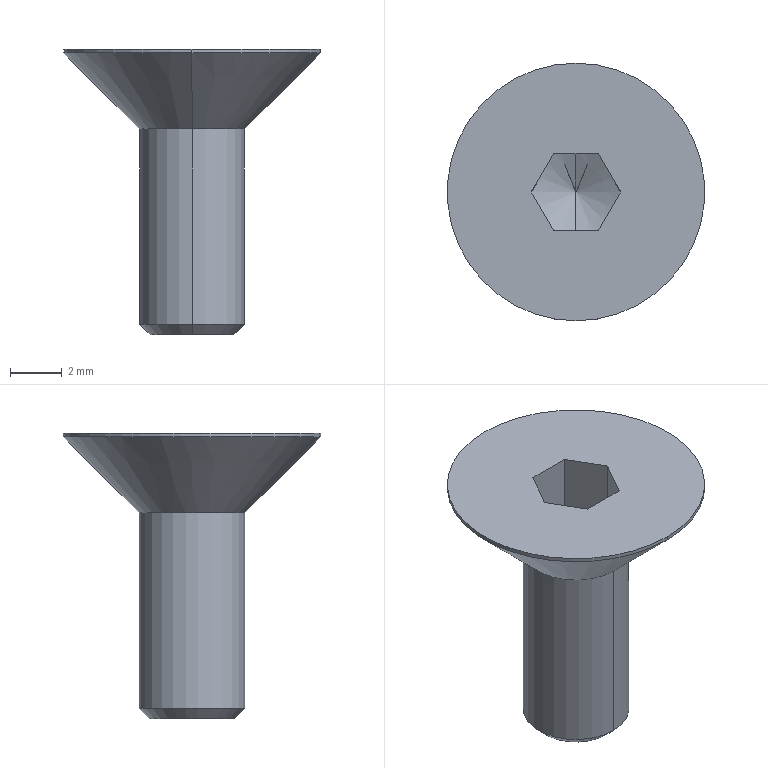Part | STEP file | Flat-head stainless hex socket screw_M5_8 | 1 solid | 24 faces | box 10 x 10 x 11.1 mm | volume 211.569 mm3 | plane 14 | cone 6 | cylinder 4 | commonest cylinder face diameters 4.1 x2 10 x2
STEP:
#1=CARTESIAN_POINT('',(0.,0.,0.));
#2=DIRECTION('',(0.,0.,1.));
#3=DIRECTION('',(1.,0.,0.));
#4=AXIS2_PLACEMENT_3D('',#1,#2,#3);
#5=CARTESIAN_POINT('',(0.,-5.,3.1));
#6=VERTEX_POINT('',#5);
#7=CARTESIAN_POINT('',(0.,5.,3.1));
#8=VERTEX_POINT('',#7);
#9=CARTESIAN_POINT('',(0.,0.,3.1));
#10=DIRECTION('',(0.,0.,1.));
#11=DIRECTION('',(0.,1.,0.));
#12=AXIS2_PLACEMENT_3D('',#9,#10,#11);
#13=CIRCLE('',#12,5.);
#14=CARTESIAN_POINT('',(0.,0.,3.1));
#15=DIRECTION('',(0.,0.,-1.));
#16=DIRECTION('',(0.,1.,0.));
#17=AXIS2_PLACEMENT_3D('',#14,#15,#16);
#18=CYLINDRICAL_SURFACE('',#17,5.);
#19=CARTESIAN_POINT('',(6.283,0.));
#20=DIRECTION('',(-1.,0.));
#21=VECTOR('',#20,1.);
#22=LINE('',#19,#21);
#23=(GEOMETRIC_REPRESENTATION_CONTEXT(2)PARAMETRIC_REPRESENTATION_CONTEXT()REPRESENTATION_CONTEXT('',''));
#24=DEFINITIONAL_REPRESENTATION('',(#22),#23);
#25=PCURVE('',#18,#24);
#26=CARTESIAN_POINT('',(0.,0.,3.1));
#27=DIRECTION('',(0.,0.,1.));
#28=DIRECTION('',(0.,-1.,0.));
#29=AXIS2_PLACEMENT_3D('',#26,#27,#28);
#30=PLANE('',#29);
#31=CARTESIAN_POINT('',(0.,0.));
#32=DIRECTION('',(-1.,0.));
#33=AXIS2_PLACEMENT_2D('',#31,#32);
#34=CIRCLE('',#33,5.);
#35=(GEOMETRIC_REPRESENTATION_CONTEXT(2)PARAMETRIC_REPRESENTATION_CONTEXT()REPRESENTATION_CONTEXT('',''));
#36=DEFINITIONAL_REPRESENTATION('',(#34),#35);
#37=PCURVE('',#30,#36);
#38=SURFACE_CURVE('',#13,(#25,#37),.PCURVE_S1.);
#39=EDGE_CURVE('',#6,#8,#38,.T.);
#40=ORIENTED_EDGE('',*,*,#39,.F.);
#41=CARTESIAN_POINT('',(0.,-5.,2.95));
#42=VERTEX_POINT('',#41);
#43=CARTESIAN_POINT('',(0.,-5.,3.1));
#44=DIRECTION('',(0.,0.,-1.));
#45=VECTOR('',#44,1.);
#46=LINE('',#43,#45);
#47=CARTESIAN_POINT('',(3.142,0.));
#48=DIRECTION('',(0.,1.));
#49=VECTOR('',#48,1.);
#50=LINE('',#47,#49);
#51=(GEOMETRIC_REPRESENTATION_CONTEXT(2)PARAMETRIC_REPRESENTATION_CONTEXT()REPRESENTATION_CONTEXT('',''));
#52=DEFINITIONAL_REPRESENTATION('',(#50),#51);
#53=PCURVE('',#18,#52);
#54=CARTESIAN_POINT('',(0.,0.,3.1));
#55=DIRECTION('',(0.,0.,-1.));
#56=DIRECTION('',(0.,1.,0.));
#57=AXIS2_PLACEMENT_3D('',#54,#55,#56);
#58=CYLINDRICAL_SURFACE('',#57,5.);
#59=CARTESIAN_POINT('',(3.142,0.));
#60=DIRECTION('',(0.,1.));
#61=VECTOR('',#60,1.);
#62=LINE('',#59,#61);
#63=(GEOMETRIC_REPRESENTATION_CONTEXT(2)PARAMETRIC_REPRESENTATION_CONTEXT()REPRESENTATION_CONTEXT('',''));
#64=DEFINITIONAL_REPRESENTATION('',(#62),#63);
#65=PCURVE('',#58,#64);
#66=SURFACE_CURVE('',#46,(#53,#65),.PCURVE_S1.);
#67=EDGE_CURVE('',#6,#42,#66,.T.);
#68=ORIENTED_EDGE('',*,*,#67,.T.);
#69=CARTESIAN_POINT('',(0.,5.,2.95));
#70=VERTEX_POINT('',#69);
#71=CARTESIAN_POINT('',(0.,0.,2.95));
#72=DIRECTION('',(0.,0.,1.));
#73=DIRECTION('',(0.,1.,0.));
#74=AXIS2_PLACEMENT_3D('',#71,#72,#73);
#75=CIRCLE('',#74,5.);
#76=CARTESIAN_POINT('',(6.283,0.15));
#77=DIRECTION('',(-1.,0.));
#78=VECTOR('',#77,1.);
#79=LINE('',#76,#78);
#80=(GEOMETRIC_REPRESENTATION_CONTEXT(2)PARAMETRIC_REPRESENTATION_CONTEXT()REPRESENTATION_CONTEXT('',''));
#81=DEFINITIONAL_REPRESENTATION('',(#79),#80);
#82=PCURVE('',#18,#81);
#83=CARTESIAN_POINT('',(0.,0.,2.95));
#84=DIRECTION('',(0.,0.,1.));
#85=DIRECTION('',(0.,-1.,0.));
#86=AXIS2_PLACEMENT_3D('',#83,#84,#85);
#87=CONICAL_SURFACE('',#86,5.,0.7854);
#88=CARTESIAN_POINT('',(-3.142,0.));
#89=DIRECTION('',(1.,0.));
#90=VECTOR('',#89,1.);
#91=LINE('',#88,#90);
#92=(GEOMETRIC_REPRESENTATION_CONTEXT(2)PARAMETRIC_REPRESENTATION_CONTEXT()REPRESENTATION_CONTEXT('',''));
#93=DEFINITIONAL_REPRESENTATION('',(#91),#92);
#94=PCURVE('',#87,#93);
#95=SURFACE_CURVE('',#75,(#82,#94),.PCURVE_S1.);
#96=EDGE_CURVE('',#42,#70,#95,.T.);
#97=ORIENTED_EDGE('',*,*,#96,.T.);
#98=CARTESIAN_POINT('',(0.,5.,3.1));
#99=DIRECTION('',(0.,0.,-1.));
#100=VECTOR('',#99,1.);
#101=LINE('',#98,#100);
#102=CARTESIAN_POINT('',(0.,0.));
#103=DIRECTION('',(0.,1.));
#104=VECTOR('',#103,1.);
#105=LINE('',#102,#104);
#106=(GEOMETRIC_REPRESENTATION_CONTEXT(2)PARAMETRIC_REPRESENTATION_CONTEXT()REPRESENTATION_CONTEXT('',''));
#107=DEFINITIONAL_REPRESENTATION('',(#105),#106);
#108=PCURVE('',#18,#107);
#109=CARTESIAN_POINT('',(6.283,0.));
#110=DIRECTION('',(0.,1.));
#111=VECTOR('',#110,1.);
#112=LINE('',#109,#111);
#113=(GEOMETRIC_REPRESENTATION_CONTEXT(2)PARAMETRIC_REPRESENTATION_CONTEXT()REPRESENTATION_CONTEXT('',''));
#114=DEFINITIONAL_REPRESENTATION('',(#112),#113);
#115=PCURVE('',#58,#114);
#116=SURFACE_CURVE('',#101,(#108,#115),.PCURVE_S1.);
#117=EDGE_CURVE('',#8,#70,#116,.T.);
#118=ORIENTED_EDGE('',*,*,#117,.F.);
#119=EDGE_LOOP('',(#40,#68,#97,#118));
#120=FACE_BOUND('',#119,.T.);
#121=ADVANCED_FACE('',(#120),#18,.T.);
#122=CARTESIAN_POINT('',(0.,-2.05,0.));
#123=VERTEX_POINT('',#122);
#124=CARTESIAN_POINT('',(0.,2.05,0.));
#125=VERTEX_POINT('',#124);
#126=CARTESIAN_POINT('',(0.,0.,0.));
#127=DIRECTION('',(0.,0.,1.));
#128=DIRECTION('',(1.,0.,0.));
#129=AXIS2_PLACEMENT_3D('',#126,#127,#128);
#130=CIRCLE('',#129,2.05);
#131=CARTESIAN_POINT('',(-4.712,-2.95));
#132=DIRECTION('',(1.,0.));
#133=VECTOR('',#132,1.);
#134=LINE('',#131,#133);
#135=(GEOMETRIC_REPRESENTATION_CONTEXT(2)PARAMETRIC_REPRESENTATION_CONTEXT()REPRESENTATION_CONTEXT('',''));
#136=DEFINITIONAL_REPRESENTATION('',(#134),#135);
#137=PCURVE('',#87,#136);
#138=CARTESIAN_POINT('',(0.,0.,-8.));
#139=DIRECTION('',(0.,0.,1.));
#140=DIRECTION('',(0.,-1.,0.));
#141=AXIS2_PLACEMENT_3D('',#138,#139,#140);
#142=CYLINDRICAL_SURFACE('',#141,2.05);
#143=CARTESIAN_POINT('',(-4.712,8.));
#144=DIRECTION('',(1.,0.));
#145=VECTOR('',#144,1.);
#146=LINE('',#143,#145);
#147=(GEOMETRIC_REPRESENTATION_CONTEXT(2)PARAMETRIC_REPRESENTATION_CONTEXT()REPRESENTATION_CONTEXT('',''));
#148=DEFINITIONAL_REPRESENTATION('',(#146),#147);
#149=PCURVE('',#142,#148);
#150=SURFACE_CURVE('',#130,(#137,#149),.PCURVE_S1.);
#151=EDGE_CURVE('',#123,#125,#150,.T.);
#152=ORIENTED_EDGE('',*,*,#151,.T.);
#153=CARTESIAN_POINT('',(0.,5.,2.95));
#154=DIRECTION('',(0.,0.7071,0.7071));
#155=VECTOR('',#154,1.);
#156=LINE('',#153,#155);
#157=CARTESIAN_POINT('',(3.142,0.));
#158=DIRECTION('',(0.,1.));
#159=VECTOR('',#158,1.);
#160=LINE('',#157,#159);
#161=(GEOMETRIC_REPRESENTATION_CONTEXT(2)PARAMETRIC_REPRESENTATION_CONTEXT()REPRESENTATION_CONTEXT('',''));
#162=DEFINITIONAL_REPRESENTATION('',(#160),#161);
#163=PCURVE('',#87,#162);
#164=CARTESIAN_POINT('',(0.,0.,2.95));
#165=DIRECTION('',(0.,0.,1.));
#166=DIRECTION('',(0.,-1.,0.));
#167=AXIS2_PLACEMENT_3D('',#164,#165,#166);
#168=CONICAL_SURFACE('',#167,5.,0.7854);
#169=CARTESIAN_POINT('',(3.142,0.));
#170=DIRECTION('',(0.,1.));
#171=VECTOR('',#170,1.);
#172=LINE('',#169,#171);
#173=(GEOMETRIC_REPRESENTATION_CONTEXT(2)PARAMETRIC_REPRESENTATION_CONTEXT()REPRESENTATION_CONTEXT('',''));
#174=DEFINITIONAL_REPRESENTATION('',(#172),#173);
#175=PCURVE('',#168,#174);
#176=SURFACE_CURVE('',#156,(#163,#175),.PCURVE_S1.);
#177=EDGE_CURVE('',#125,#70,#176,.T.);
#178=ORIENTED_EDGE('',*,*,#177,.T.);
#179=ORIENTED_EDGE('',*,*,#96,.F.);
#180=CARTESIAN_POINT('',(0.,-5.,2.95));
#181=DIRECTION('',(0.,-0.7071,0.7071));
#182=VECTOR('',#181,1.);
#183=LINE('',#180,#182);
#184=CARTESIAN_POINT('',(0.,0.));
#185=DIRECTION('',(0.,1.));
#186=VECTOR('',#185,1.);
#187=LINE('',#184,#186);
#188=(GEOMETRIC_REPRESENTATION_CONTEXT(2)PARAMETRIC_REPRESENTATION_CONTEXT()REPRESENTATION_CONTEXT('',''));
#189=DEFINITIONAL_REPRESENTATION('',(#187),#188);
#190=PCURVE('',#87,#189);
#191=CARTESIAN_POINT('',(6.283,0.));
#192=DIRECTION('',(0.,1.));
#193=VECTOR('',#192,1.);
#194=LINE('',#191,#193);
#195=(GEOMETRIC_REPRESENTATION_CONTEXT(2)PARAMETRIC_REPRESENTATION_CONTEXT()REPRESENTATION_CONTEXT('',''));
#196=DEFINITIONAL_REPRESENTATION('',(#194),#195);
#197=PCURVE('',#168,#196);
#198=SURFACE_CURVE('',#183,(#190,#197),.PCURVE_S1.);
#199=EDGE_CURVE('',#123,#42,#198,.T.);
#200=ORIENTED_EDGE('',*,*,#199,.F.);
#201=EDGE_LOOP('',(#152,#178,#179,#200));
#202=FACE_BOUND('',#201,.T.);
#203=ADVANCED_FACE('',(#202),#87,.T.);
#204=CARTESIAN_POINT('',(0.,-2.05,-7.59));
#205=VERTEX_POINT('',#204);
#206=CARTESIAN_POINT('',(0.,2.05,-7.59));
#207=VERTEX_POINT('',#206);
#208=CARTESIAN_POINT('',(0.,0.,-7.59));
#209=DIRECTION('',(0.,0.,1.));
#210=DIRECTION('',(0.,-1.,0.));
#211=AXIS2_PLACEMENT_3D('',#208,#209,#210);
#212=CIRCLE('',#211,2.05);
#213=CARTESIAN_POINT('',(0.,0.41));
#214=DIRECTION('',(1.,0.));
#215=VECTOR('',#214,1.);
#216=LINE('',#213,#215);
#217=(GEOMETRIC_REPRESENTATION_CONTEXT(2)PARAMETRIC_REPRESENTATION_CONTEXT()REPRESENTATION_CONTEXT('',''));
#218=DEFINITIONAL_REPRESENTATION('',(#216),#217);
#219=PCURVE('',#142,#218);
#220=CARTESIAN_POINT('',(0.,0.,-7.59));
#221=DIRECTION('',(0.,0.,1.));
#222=DIRECTION('',(0.,-1.,0.));
#223=AXIS2_PLACEMENT_3D('',#220,#221,#222);
#224=CONICAL_SURFACE('',#223,2.05,0.7854);
#225=CARTESIAN_POINT('',(0.,0.));
#226=DIRECTION('',(1.,0.));
#227=VECTOR('',#226,1.);
#228=LINE('',#225,#227);
#229=(GEOMETRIC_REPRESENTATION_CONTEXT(2)PARAMETRIC_REPRESENTATION_CONTEXT()REPRESENTATION_CONTEXT('',''));
#230=DEFINITIONAL_REPRESENTATION('',(#228),#229);
#231=PCURVE('',#224,#230);
#232=SURFACE_CURVE('',#212,(#219,#231),.PCURVE_S1.);
#233=EDGE_CURVE('',#205,#207,#232,.T.);
#234=ORIENTED_EDGE('',*,*,#233,.T.);
#235=CARTESIAN_POINT('',(0.,2.05,-8.));
#236=DIRECTION('',(0.,0.,1.));
#237=VECTOR('',#236,1.);
#238=LINE('',#235,#237);
#239=CARTESIAN_POINT('',(3.142,0.));
#240=DIRECTION('',(0.,1.));
#241=VECTOR('',#240,1.);
#242=LINE('',#239,#241);
#243=(GEOMETRIC_REPRESENTATION_CONTEXT(2)PARAMETRIC_REPRESENTATION_CONTEXT()REPRESENTATION_CONTEXT('',''));
#244=DEFINITIONAL_REPRESENTATION('',(#242),#243);
#245=PCURVE('',#142,#244);
#246=CARTESIAN_POINT('',(0.,0.,-8.));
#247=DIRECTION('',(0.,0.,1.));
#248=DIRECTION('',(0.,-1.,0.));
#249=AXIS2_PLACEMENT_3D('',#246,#247,#248);
#250=CYLINDRICAL_SURFACE('',#249,2.05);
#251=CARTESIAN_POINT('',(3.142,0.));
#252=DIRECTION('',(0.,1.));
#253=VECTOR('',#252,1.);
#254=LINE('',#251,#253);
#255=(GEOMETRIC_REPRESENTATION_CONTEXT(2)PARAMETRIC_REPRESENTATION_CONTEXT()REPRESENTATION_CONTEXT('',''));
#256=DEFINITIONAL_REPRESENTATION('',(#254),#255);
#257=PCURVE('',#250,#256);
#258=SURFACE_CURVE('',#238,(#245,#257),.PCURVE_S1.);
#259=EDGE_CURVE('',#207,#125,#258,.T.);
#260=ORIENTED_EDGE('',*,*,#259,.T.);
#261=ORIENTED_EDGE('',*,*,#151,.F.);
#262=CARTESIAN_POINT('',(0.,-2.05,-8.));
#263=DIRECTION('',(0.,0.,1.));
#264=VECTOR('',#263,1.);
#265=LINE('',#262,#264);
#266=CARTESIAN_POINT('',(0.,0.));
#267=DIRECTION('',(0.,1.));
#268=VECTOR('',#267,1.);
#269=LINE('',#266,#268);
#270=(GEOMETRIC_REPRESENTATION_CONTEXT(2)PARAMETRIC_REPRESENTATION_CONTEXT()REPRESENTATION_CONTEXT('',''));
#271=DEFINITIONAL_REPRESENTATION('',(#269),#270);
#272=PCURVE('',#142,#271);
#273=CARTESIAN_POINT('',(6.283,0.));
#274=DIRECTION('',(0.,1.));
#275=VECTOR('',#274,1.);
#276=LINE('',#273,#275);
#277=(GEOMETRIC_REPRESENTATION_CONTEXT(2)PARAMETRIC_REPRESENTATION_CONTEXT()REPRESENTATION_CONTEXT('',''));
#278=DEFINITIONAL_REPRESENTATION('',(#276),#277);
#279=PCURVE('',#250,#278);
#280=SURFACE_CURVE('',#265,(#272,#279),.PCURVE_S1.);
#281=EDGE_CURVE('',#205,#123,#280,.T.);
#282=ORIENTED_EDGE('',*,*,#281,.F.);
#283=EDGE_LOOP('',(#234,#260,#261,#282));
#284=FACE_BOUND('',#283,.T.);
#285=ADVANCED_FACE('',(#284),#142,.T.);
#286=CARTESIAN_POINT('',(0.,-1.64,-8.));
#287=VERTEX_POINT('',#286);
#288=CARTESIAN_POINT('',(0.,1.64,-8.));
#289=VERTEX_POINT('',#288);
#290=CARTESIAN_POINT('',(0.,0.,-8.));
#291=DIRECTION('',(0.,0.,1.));
#292=DIRECTION('',(0.,-1.,0.));
#293=AXIS2_PLACEMENT_3D('',#290,#291,#292);
#294=CIRCLE('',#293,1.64);
#295=CARTESIAN_POINT('',(0.,-0.41));
#296=DIRECTION('',(1.,0.));
#297=VECTOR('',#296,1.);
#298=LINE('',#295,#297);
#299=(GEOMETRIC_REPRESENTATION_CONTEXT(2)PARAMETRIC_REPRESENTATION_CONTEXT()REPRESENTATION_CONTEXT('',''));
#300=DEFINITIONAL_REPRESENTATION('',(#298),#299);
#301=PCURVE('',#224,#300);
#302=CARTESIAN_POINT('',(0.,0.,-8.));
#303=DIRECTION('',(0.,0.,-1.));
#304=DIRECTION('',(0.,1.,0.));
#305=AXIS2_PLACEMENT_3D('',#302,#303,#304);
#306=PLANE('',#305);
#307=CARTESIAN_POINT('',(-1.64,0.));
#308=CARTESIAN_POINT('',(-1.64,2.841));
#309=CARTESIAN_POINT('',(0.82,1.42));
#310=CARTESIAN_POINT('',(3.28,0.));
#311=CARTESIAN_POINT('',(0.82,-1.42));
#312=CARTESIAN_POINT('',(-1.64,-2.841));
#313=CARTESIAN_POINT('',(-1.64,0.));
#314=(BOUNDED_CURVE()B_SPLINE_CURVE(2,(#307,#308,#309,#310,#311,#312,#313),.UNSPECIFIED.,.T.,.F.)B_SPLINE_CURVE_WITH_KNOTS((1,2,2,2,2,1),(-2.094,0.,2.094,4.189,6.283,8.378),.UNSPECIFIED.)CURVE()GEOMETRIC_REPRESENTATION_ITEM()RATIONAL_B_SPLINE_CURVE((1.,0.5,1.,0.5,1.,0.5,1.))REPRESENTATION_ITEM(''));
#315=(GEOMETRIC_REPRESENTATION_CONTEXT(2)PARAMETRIC_REPRESENTATION_CONTEXT()REPRESENTATION_CONTEXT('',''));
#316=DEFINITIONAL_REPRESENTATION('',(#314),#315);
#317=PCURVE('',#306,#316);
#318=SURFACE_CURVE('',#294,(#301,#317),.PCURVE_S1.);
#319=EDGE_CURVE('',#287,#289,#318,.T.);
#320=ORIENTED_EDGE('',*,*,#319,.T.);
#321=CARTESIAN_POINT('',(0.,2.05,-7.59));
#322=DIRECTION('',(0.,0.7071,0.7071));
#323=VECTOR('',#322,1.);
#324=LINE('',#321,#323);
#325=CARTESIAN_POINT('',(3.142,0.));
#326=DIRECTION('',(0.,1.));
#327=VECTOR('',#326,1.);
#328=LINE('',#325,#327);
#329=(GEOMETRIC_REPRESENTATION_CONTEXT(2)PARAMETRIC_REPRESENTATION_CONTEXT()REPRESENTATION_CONTEXT('',''));
#330=DEFINITIONAL_REPRESENTATION('',(#328),#329);
#331=PCURVE('',#224,#330);
#332=CARTESIAN_POINT('',(0.,0.,-7.59));
#333=DIRECTION('',(0.,0.,1.));
#334=DIRECTION('',(0.,-1.,0.));
#335=AXIS2_PLACEMENT_3D('',#332,#333,#334);
#336=CONICAL_SURFACE('',#335,2.05,0.7854);
#337=CARTESIAN_POINT('',(3.142,0.));
#338=DIRECTION('',(0.,1.));
#339=VECTOR('',#338,1.);
#340=LINE('',#337,#339);
#341=(GEOMETRIC_REPRESENTATION_CONTEXT(2)PARAMETRIC_REPRESENTATION_CONTEXT()REPRESENTATION_CONTEXT('',''));
#342=DEFINITIONAL_REPRESENTATION('',(#340),#341);
#343=PCURVE('',#336,#342);
#344=SURFACE_CURVE('',#324,(#331,#343),.PCURVE_S1.);
#345=EDGE_CURVE('',#289,#207,#344,.T.);
#346=ORIENTED_EDGE('',*,*,#345,.T.);
#347=ORIENTED_EDGE('',*,*,#233,.F.);
#348=CARTESIAN_POINT('',(0.,-2.05,-7.59));
#349=DIRECTION('',(0.,-0.7071,0.7071));
#350=VECTOR('',#349,1.);
#351=LINE('',#348,#350);
#352=CARTESIAN_POINT('',(0.,0.));
#353=DIRECTION('',(0.,1.));
#354=VECTOR('',#353,1.);
#355=LINE('',#352,#354);
#356=(GEOMETRIC_REPRESENTATION_CONTEXT(2)PARAMETRIC_REPRESENTATION_CONTEXT()REPRESENTATION_CONTEXT('',''));
#357=DEFINITIONAL_REPRESENTATION('',(#355),#356);
#358=PCURVE('',#224,#357);
#359=CARTESIAN_POINT('',(6.283,0.));
#360=DIRECTION('',(0.,1.));
#361=VECTOR('',#360,1.);
#362=LINE('',#359,#361);
#363=(GEOMETRIC_REPRESENTATION_CONTEXT(2)PARAMETRIC_REPRESENTATION_CONTEXT()REPRESENTATION_CONTEXT('',''));
#364=DEFINITIONAL_REPRESENTATION('',(#362),#363);
#365=PCURVE('',#336,#364);
#366=SURFACE_CURVE('',#351,(#358,#365),.PCURVE_S1.);
#367=EDGE_CURVE('',#287,#205,#366,.T.);
#368=ORIENTED_EDGE('',*,*,#367,.F.);
#369=EDGE_LOOP('',(#320,#346,#347,#368));
#370=FACE_BOUND('',#369,.T.);
#371=ADVANCED_FACE('',(#370),#224,.T.);
#372=CARTESIAN_POINT('',(-0.866,-1.5,0.));
#373=VERTEX_POINT('',#372);
#374=CARTESIAN_POINT('',(0.,-1.732,0.));
#375=VERTEX_POINT('',#374);
#376=CARTESIAN_POINT('',(0.,0.,0.));
#377=DIRECTION('',(0.,0.,1.));
#378=DIRECTION('',(0.,-1.,0.));
#379=AXIS2_PLACEMENT_3D('',#376,#377,#378);
#380=CIRCLE('',#379,1.732);
#381=CARTESIAN_POINT('',(0.,0.,0.));
#382=DIRECTION('',(0.,0.,1.));
#383=DIRECTION('',(0.,-1.,0.));
#384=AXIS2_PLACEMENT_3D('',#381,#382,#383);
#385=CONICAL_SURFACE('',#384,1.732,1.134);
#386=CARTESIAN_POINT('',(0.,0.));
#387=DIRECTION('',(1.,0.));
#388=VECTOR('',#387,1.);
#389=LINE('',#386,#388);
#390=(GEOMETRIC_REPRESENTATION_CONTEXT(2)PARAMETRIC_REPRESENTATION_CONTEXT()REPRESENTATION_CONTEXT('',''));
#391=DEFINITIONAL_REPRESENTATION('',(#389),#390);
#392=PCURVE('',#385,#391);
#393=CARTESIAN_POINT('',(1.732,0.,0.));
#394=DIRECTION('',(0.,0.,1.));
#395=DIRECTION('',(0.,-1.,0.));
#396=AXIS2_PLACEMENT_3D('',#393,#394,#395);
#397=PLANE('',#396);
#398=CARTESIAN_POINT('',(0.,-1.732));
#399=DIRECTION('',(1.,0.));
#400=AXIS2_PLACEMENT_2D('',#398,#399);
#401=CIRCLE('',#400,1.732);
#402=(GEOMETRIC_REPRESENTATION_CONTEXT(2)PARAMETRIC_REPRESENTATION_CONTEXT()REPRESENTATION_CONTEXT('',''));
#403=DEFINITIONAL_REPRESENTATION('',(#401),#402);
#404=PCURVE('',#397,#403);
#405=SURFACE_CURVE('',#380,(#392,#404),.PCURVE_S1.);
#406=EDGE_CURVE('',#373,#375,#405,.T.);
#407=ORIENTED_EDGE('',*,*,#406,.F.);
#408=CARTESIAN_POINT('',(-1.732,0.,0.));
#409=VERTEX_POINT('',#408);
#410=CARTESIAN_POINT('',(0.,0.,0.));
#411=DIRECTION('',(0.,0.,-1.));
#412=DIRECTION('',(0.,-1.,0.));
#413=AXIS2_PLACEMENT_3D('',#410,#411,#412);
#414=CIRCLE('',#413,1.732);
#415=CARTESIAN_POINT('',(6.283,0.));
#416=DIRECTION('',(-1.,0.));
#417=VECTOR('',#416,1.);
#418=LINE('',#415,#417);
#419=(GEOMETRIC_REPRESENTATION_CONTEXT(2)PARAMETRIC_REPRESENTATION_CONTEXT()REPRESENTATION_CONTEXT('',''));
#420=DEFINITIONAL_REPRESENTATION('',(#418),#419);
#421=PCURVE('',#385,#420);
#422=CARTESIAN_POINT('',(1.732,0.,0.));
#423=DIRECTION('',(0.,0.,1.));
#424=DIRECTION('',(0.,-1.,0.));
#425=AXIS2_PLACEMENT_3D('',#422,#423,#424);
#426=PLANE('',#425);
#427=CARTESIAN_POINT('',(1.732,-1.732));
#428=CARTESIAN_POINT('',(1.732,-4.732));
#429=CARTESIAN_POINT('',(-0.866,-3.232));
#430=CARTESIAN_POINT('',(-3.464,-1.732));
#431=CARTESIAN_POINT('',(-0.866,-0.2321));
#432=CARTESIAN_POINT('',(1.732,1.268));
#433=CARTESIAN_POINT('',(1.732,-1.732));
#434=(BOUNDED_CURVE()B_SPLINE_CURVE(2,(#427,#428,#429,#430,#431,#432,#433),.UNSPECIFIED.,.T.,.F.)B_SPLINE_CURVE_WITH_KNOTS((1,2,2,2,2,1),(-2.094,0.,2.094,4.189,6.283,8.378),.UNSPECIFIED.)CURVE()GEOMETRIC_REPRESENTATION_ITEM()RATIONAL_B_SPLINE_CURVE((1.,0.5,1.,0.5,1.,0.5,1.))REPRESENTATION_ITEM(''));
#435=(GEOMETRIC_REPRESENTATION_CONTEXT(2)PARAMETRIC_REPRESENTATION_CONTEXT()REPRESENTATION_CONTEXT('',''));
#436=DEFINITIONAL_REPRESENTATION('',(#434),#435);
#437=PCURVE('',#426,#436);
#438=SURFACE_CURVE('',#414,(#421,#437),.PCURVE_S1.);
#439=EDGE_CURVE('',#373,#409,#438,.T.);
#440=ORIENTED_EDGE('',*,*,#439,.T.);
#441=CARTESIAN_POINT('',(-0.866,1.5,0.));
#442=VERTEX_POINT('',#441);
#443=CARTESIAN_POINT('',(0.,0.,0.));
#444=DIRECTION('',(0.,0.,-1.));
#445=DIRECTION('',(0.,-1.,0.));
#446=AXIS2_PLACEMENT_3D('',#443,#444,#445);
#447=CIRCLE('',#446,1.732);
#448=CARTESIAN_POINT('',(6.283,0.));
#449=DIRECTION('',(-1.,0.));
#450=VECTOR('',#449,1.);
#451=LINE('',#448,#450);
#452=(GEOMETRIC_REPRESENTATION_CONTEXT(2)PARAMETRIC_REPRESENTATION_CONTEXT()REPRESENTATION_CONTEXT('',''));
#453=DEFINITIONAL_REPRESENTATION('',(#451),#452);
#454=PCURVE('',#385,#453);
#455=CARTESIAN_POINT('',(1.732,0.,0.));
#456=DIRECTION('',(0.,0.,1.));
#457=DIRECTION('',(0.,-1.,0.));
#458=AXIS2_PLACEMENT_3D('',#455,#456,#457);
#459=PLANE('',#458);
#460=CARTESIAN_POINT('',(1.732,-1.732));
#461=CARTESIAN_POINT('',(1.732,-4.732));
#462=CARTESIAN_POINT('',(-0.866,-3.232));
#463=CARTESIAN_POINT('',(-3.464,-1.732));
#464=CARTESIAN_POINT('',(-0.866,-0.2321));
#465=CARTESIAN_POINT('',(1.732,1.268));
#466=CARTESIAN_POINT('',(1.732,-1.732));
#467=(BOUNDED_CURVE()B_SPLINE_CURVE(2,(#460,#461,#462,#463,#464,#465,#466),.UNSPECIFIED.,.T.,.F.)B_SPLINE_CURVE_WITH_KNOTS((1,2,2,2,2,1),(-2.094,0.,2.094,4.189,6.283,8.378),.UNSPECIFIED.)CURVE()GEOMETRIC_REPRESENTATION_ITEM()RATIONAL_B_SPLINE_CURVE((1.,0.5,1.,0.5,1.,0.5,1.))REPRESENTATION_ITEM(''));
#468=(GEOMETRIC_REPRESENTATION_CONTEXT(2)PARAMETRIC_REPRESENTATION_CONTEXT()REPRESENTATION_CONTEXT('',''));
#469=DEFINITIONAL_REPRESENTATION('',(#467),#468);
#470=PCURVE('',#459,#469);
#471=SURFACE_CURVE('',#447,(#454,#470),.PCURVE_S1.);
#472=EDGE_CURVE('',#409,#442,#471,.T.);
#473=ORIENTED_EDGE('',*,*,#472,.T.);
#474=CARTESIAN_POINT('',(0.,1.732,0.));
#475=VERTEX_POINT('',#474);
#476=CARTESIAN_POINT('',(0.,0.,0.));
#477=DIRECTION('',(0.,0.,-1.));
#478=DIRECTION('',(0.,-1.,0.));
#479=AXIS2_PLACEMENT_3D('',#476,#477,#478);
#480=CIRCLE('',#479,1.732);
#481=CARTESIAN_POINT('',(6.283,0.));
#482=DIRECTION('',(-1.,0.));
#483=VECTOR('',#482,1.);
#484=LINE('',#481,#483);
#485=(GEOMETRIC_REPRESENTATION_CONTEXT(2)PARAMETRIC_REPRESENTATION_CONTEXT()REPRESENTATION_CONTEXT('',''));
#486=DEFINITIONAL_REPRESENTATION('',(#484),#485);
#487=PCURVE('',#385,#486);
#488=CARTESIAN_POINT('',(1.732,0.,0.));
#489=DIRECTION('',(0.,0.,1.));
#490=DIRECTION('',(0.,-1.,0.));
#491=AXIS2_PLACEMENT_3D('',#488,#489,#490);
#492=PLANE('',#491);
#493=CARTESIAN_POINT('',(1.732,-1.732));
#494=CARTESIAN_POINT('',(1.732,-4.732));
#495=CARTESIAN_POINT('',(-0.866,-3.232));
#496=CARTESIAN_POINT('',(-3.464,-1.732));
#497=CARTESIAN_POINT('',(-0.866,-0.2321));
#498=CARTESIAN_POINT('',(1.732,1.268));
#499=CARTESIAN_POINT('',(1.732,-1.732));
#500=(BOUNDED_CURVE()B_SPLINE_CURVE(2,(#493,#494,#495,#496,#497,#498,#499),.UNSPECIFIED.,.T.,.F.)B_SPLINE_CURVE_WITH_KNOTS((1,2,2,2,2,1),(-2.094,0.,2.094,4.189,6.283,8.378),.UNSPECIFIED.)CURVE()GEOMETRIC_REPRESENTATION_ITEM()RATIONAL_B_SPLINE_CURVE((1.,0.5,1.,0.5,1.,0.5,1.))REPRESENTATION_ITEM(''));
#501=(GEOMETRIC_REPRESENTATION_CONTEXT(2)PARAMETRIC_REPRESENTATION_CONTEXT()REPRESENTATION_CONTEXT('',''));
#502=DEFINITIONAL_REPRESENTATION('',(#500),#501);
#503=PCURVE('',#492,#502);
#504=SURFACE_CURVE('',#480,(#487,#503),.PCURVE_S1.);
#505=EDGE_CURVE('',#442,#475,#504,.T.);
#506=ORIENTED_EDGE('',*,*,#505,.T.);
#507=CARTESIAN_POINT('',(0.,0.,-0.8077));
#508=VERTEX_POINT('',#507);
#509=CARTESIAN_POINT('',(0.,1.732,0.));
#510=DIRECTION('',(0.,0.9063,0.4226));
#511=VECTOR('',#510,1.);
#512=LINE('',#509,#511);
#513=CARTESIAN_POINT('',(3.142,0.));
#514=DIRECTION('',(0.,1.));
#515=VECTOR('',#514,1.);
#516=LINE('',#513,#515);
#517=(GEOMETRIC_REPRESENTATION_CONTEXT(2)PARAMETRIC_REPRESENTATION_CONTEXT()REPRESENTATION_CONTEXT('',''));
#518=DEFINITIONAL_REPRESENTATION('',(#516),#517);
#519=PCURVE('',#385,#518);
#520=CARTESIAN_POINT('',(0.,0.,0.));
#521=DIRECTION('',(0.,0.,1.));
#522=DIRECTION('',(0.,-1.,0.));
#523=AXIS2_PLACEMENT_3D('',#520,#521,#522);
#524=CONICAL_SURFACE('',#523,1.732,1.134);
#525=CARTESIAN_POINT('',(3.142,0.));
#526=DIRECTION('',(0.,1.));
#527=VECTOR('',#526,1.);
#528=LINE('',#525,#527);
#529=(GEOMETRIC_REPRESENTATION_CONTEXT(2)PARAMETRIC_REPRESENTATION_CONTEXT()REPRESENTATION_CONTEXT('',''));
#530=DEFINITIONAL_REPRESENTATION('',(#528),#529);
#531=PCURVE('',#524,#530);
#532=SURFACE_CURVE('',#512,(#519,#531),.PCURVE_S1.);
#533=EDGE_CURVE('',#508,#475,#532,.T.);
#534=ORIENTED_EDGE('',*,*,#533,.F.);
#535=CARTESIAN_POINT('',(0.,-1.732,0.));
#536=DIRECTION('',(0.,-0.9063,0.4226));
#537=VECTOR('',#536,1.);
#538=LINE('',#535,#537);
#539=CARTESIAN_POINT('',(6.283,0.));
#540=DIRECTION('',(0.,1.));
#541=VECTOR('',#540,1.);
#542=LINE('',#539,#541);
#543=(GEOMETRIC_REPRESENTATION_CONTEXT(2)PARAMETRIC_REPRESENTATION_CONTEXT()REPRESENTATION_CONTEXT('',''));
#544=DEFINITIONAL_REPRESENTATION('',(#542),#543);
#545=PCURVE('',#385,#544);
#546=CARTESIAN_POINT('',(0.,0.));
#547=DIRECTION('',(0.,1.));
#548=VECTOR('',#547,1.);
#549=LINE('',#546,#548);
#550=(GEOMETRIC_REPRESENTATION_CONTEXT(2)PARAMETRIC_REPRESENTATION_CONTEXT()REPRESENTATION_CONTEXT('',''));
#551=DEFINITIONAL_REPRESENTATION('',(#549),#550);
#552=PCURVE('',#524,#551);
#553=SURFACE_CURVE('',#538,(#545,#552),.PCURVE_S1.);
#554=EDGE_CURVE('',#508,#375,#553,.T.);
#555=ORIENTED_EDGE('',*,*,#554,.T.);
#556=EDGE_LOOP('',(#407,#440,#473,#506,#534,#555));
#557=FACE_BOUND('',#556,.F.);
#558=ADVANCED_FACE('',(#557),#385,.F.);
#559=CARTESIAN_POINT('',(0.,0.,3.1));
#560=DIRECTION('',(0.,0.,1.));
#561=DIRECTION('',(0.,1.,0.));
#562=AXIS2_PLACEMENT_3D('',#559,#560,#561);
#563=CIRCLE('',#562,5.);
#564=CARTESIAN_POINT('',(0.,0.));
#565=DIRECTION('',(-1.,0.));
#566=AXIS2_PLACEMENT_2D('',#564,#565);
#567=CIRCLE('',#566,5.);
#568=(GEOMETRIC_REPRESENTATION_CONTEXT(2)PARAMETRIC_REPRESENTATION_CONTEXT()REPRESENTATION_CONTEXT('',''));
#569=DEFINITIONAL_REPRESENTATION('',(#567),#568);
#570=PCURVE('',#30,#569);
#571=CARTESIAN_POINT('',(6.283,0.));
#572=DIRECTION('',(-1.,0.));
#573=VECTOR('',#572,1.);
#574=LINE('',#571,#573);
#575=(GEOMETRIC_REPRESENTATION_CONTEXT(2)PARAMETRIC_REPRESENTATION_CONTEXT()REPRESENTATION_CONTEXT('',''));
#576=DEFINITIONAL_REPRESENTATION('',(#574),#575);
#577=PCURVE('',#58,#576);
#578=SURFACE_CURVE('',#563,(#570,#577),.PCURVE_S1.);
#579=EDGE_CURVE('',#8,#6,#578,.T.);
#580=ORIENTED_EDGE('',*,*,#579,.T.);
#581=ORIENTED_EDGE('',*,*,#39,.T.);
#582=EDGE_LOOP('',(#580,#581));
#583=FACE_BOUND('',#582,.T.);
#584=CARTESIAN_POINT('',(-1.732,0.,3.1));
#585=VERTEX_POINT('',#584);
#586=CARTESIAN_POINT('',(-0.866,1.5,3.1));
#587=VERTEX_POINT('',#586);
#588=CARTESIAN_POINT('',(-0.866,1.5,3.1));
#589=DIRECTION('',(0.5,0.866,0.));
#590=VECTOR('',#589,1.);
#591=LINE('',#588,#590);
#592=CARTESIAN_POINT('',(-1.5,-0.866));
#593=DIRECTION('',(-0.866,0.5));
#594=VECTOR('',#593,1.);
#595=LINE('',#592,#594);
#596=(GEOMETRIC_REPRESENTATION_CONTEXT(2)PARAMETRIC_REPRESENTATION_CONTEXT()REPRESENTATION_CONTEXT('',''));
#597=DEFINITIONAL_REPRESENTATION('',(#595),#596);
#598=PCURVE('',#30,#597);
#599=CARTESIAN_POINT('',(-0.866,1.5,0.));
#600=DIRECTION('',(-0.866,0.5,0.));
#601=DIRECTION('',(-0.5,-0.866,0.));
#602=AXIS2_PLACEMENT_3D('',#599,#600,#601);
#603=PLANE('',#602);
#604=CARTESIAN_POINT('',(0.,3.1));
#605=DIRECTION('',(-1.,0.));
#606=VECTOR('',#605,1.);
#607=LINE('',#604,#606);
#608=(GEOMETRIC_REPRESENTATION_CONTEXT(2)PARAMETRIC_REPRESENTATION_CONTEXT()REPRESENTATION_CONTEXT('',''));
#609=DEFINITIONAL_REPRESENTATION('',(#607),#608);
#610=PCURVE('',#603,#609);
#611=SURFACE_CURVE('',#591,(#598,#610),.PCURVE_S1.);
#612=EDGE_CURVE('',#585,#587,#611,.T.);
#613=ORIENTED_EDGE('',*,*,#612,.T.);
#614=CARTESIAN_POINT('',(0.866,1.5,3.1));
#615=VERTEX_POINT('',#614);
#616=CARTESIAN_POINT('',(0.,1.5,3.1));
#617=DIRECTION('',(1.,0.,0.));
#618=VECTOR('',#617,1.);
#619=LINE('',#616,#618);
#620=CARTESIAN_POINT('',(-1.5,0.));
#621=DIRECTION('',(0.,1.));
#622=VECTOR('',#621,1.);
#623=LINE('',#620,#622);
#624=(GEOMETRIC_REPRESENTATION_CONTEXT(2)PARAMETRIC_REPRESENTATION_CONTEXT()REPRESENTATION_CONTEXT('',''));
#625=DEFINITIONAL_REPRESENTATION('',(#623),#624);
#626=PCURVE('',#30,#625);
#627=CARTESIAN_POINT('',(0.866,1.5,0.));
#628=DIRECTION('',(0.,1.,0.));
#629=DIRECTION('',(-1.,0.,0.));
#630=AXIS2_PLACEMENT_3D('',#627,#628,#629);
#631=PLANE('',#630);
#632=CARTESIAN_POINT('',(0.866,3.1));
#633=DIRECTION('',(-1.,0.));
#634=VECTOR('',#633,1.);
#635=LINE('',#632,#634);
#636=(GEOMETRIC_REPRESENTATION_CONTEXT(2)PARAMETRIC_REPRESENTATION_CONTEXT()REPRESENTATION_CONTEXT('',''));
#637=DEFINITIONAL_REPRESENTATION('',(#635),#636);
#638=PCURVE('',#631,#637);
#639=SURFACE_CURVE('',#619,(#626,#638),.PCURVE_S1.);
#640=EDGE_CURVE('',#587,#615,#639,.T.);
#641=ORIENTED_EDGE('',*,*,#640,.T.);
#642=CARTESIAN_POINT('',(1.732,0.,3.1));
#643=VERTEX_POINT('',#642);
#644=CARTESIAN_POINT('',(1.732,0.,3.1));
#645=DIRECTION('',(0.5,-0.866,0.));
#646=VECTOR('',#645,1.);
#647=LINE('',#644,#646);
#648=CARTESIAN_POINT('',(0.,1.732));
#649=DIRECTION('',(0.866,0.5));
#650=VECTOR('',#649,1.);
#651=LINE('',#648,#650);
#652=(GEOMETRIC_REPRESENTATION_CONTEXT(2)PARAMETRIC_REPRESENTATION_CONTEXT()REPRESENTATION_CONTEXT('',''));
#653=DEFINITIONAL_REPRESENTATION('',(#651),#652);
#654=PCURVE('',#30,#653);
#655=CARTESIAN_POINT('',(1.732,0.,0.));
#656=DIRECTION('',(0.866,0.5,0.));
#657=DIRECTION('',(-0.5,0.866,0.));
#658=AXIS2_PLACEMENT_3D('',#655,#656,#657);
#659=PLANE('',#658);
#660=CARTESIAN_POINT('',(0.,3.1));
#661=DIRECTION('',(-1.,0.));
#662=VECTOR('',#661,1.);
#663=LINE('',#660,#662);
#664=(GEOMETRIC_REPRESENTATION_CONTEXT(2)PARAMETRIC_REPRESENTATION_CONTEXT()REPRESENTATION_CONTEXT('',''));
#665=DEFINITIONAL_REPRESENTATION('',(#663),#664);
#666=PCURVE('',#659,#665);
#667=SURFACE_CURVE('',#647,(#654,#666),.PCURVE_S1.);
#668=EDGE_CURVE('',#615,#643,#667,.T.);
#669=ORIENTED_EDGE('',*,*,#668,.T.);
#670=CARTESIAN_POINT('',(0.866,-1.5,3.1));
#671=VERTEX_POINT('',#670);
#672=CARTESIAN_POINT('',(0.866,-1.5,3.1));
#673=DIRECTION('',(-0.5,-0.866,0.));
#674=VECTOR('',#673,1.);
#675=LINE('',#672,#674);
#676=CARTESIAN_POINT('',(1.5,0.866));
#677=DIRECTION('',(0.866,-0.5));
#678=VECTOR('',#677,1.);
#679=LINE('',#676,#678);
#680=(GEOMETRIC_REPRESENTATION_CONTEXT(2)PARAMETRIC_REPRESENTATION_CONTEXT()REPRESENTATION_CONTEXT('',''));
#681=DEFINITIONAL_REPRESENTATION('',(#679),#680);
#682=PCURVE('',#30,#681);
#683=CARTESIAN_POINT('',(0.866,-1.5,0.));
#684=DIRECTION('',(0.866,-0.5,0.));
#685=DIRECTION('',(0.5,0.866,0.));
#686=AXIS2_PLACEMENT_3D('',#683,#684,#685);
#687=PLANE('',#686);
#688=CARTESIAN_POINT('',(0.,3.1));
#689=DIRECTION('',(-1.,0.));
#690=VECTOR('',#689,1.);
#691=LINE('',#688,#690);
#692=(GEOMETRIC_REPRESENTATION_CONTEXT(2)PARAMETRIC_REPRESENTATION_CONTEXT()REPRESENTATION_CONTEXT('',''));
#693=DEFINITIONAL_REPRESENTATION('',(#691),#692);
#694=PCURVE('',#687,#693);
#695=SURFACE_CURVE('',#675,(#682,#694),.PCURVE_S1.);
#696=EDGE_CURVE('',#643,#671,#695,.T.);
#697=ORIENTED_EDGE('',*,*,#696,.T.);
#698=CARTESIAN_POINT('',(-0.866,-1.5,3.1));
#699=VERTEX_POINT('',#698);
#700=CARTESIAN_POINT('',(-0.866,-1.5,3.1));
#701=DIRECTION('',(-1.,0.,0.));
#702=VECTOR('',#701,1.);
#703=LINE('',#700,#702);
#704=CARTESIAN_POINT('',(1.5,-0.866));
#705=DIRECTION('',(0.,-1.));
#706=VECTOR('',#705,1.);
#707=LINE('',#704,#706);
#708=(GEOMETRIC_REPRESENTATION_CONTEXT(2)PARAMETRIC_REPRESENTATION_CONTEXT()REPRESENTATION_CONTEXT('',''));
#709=DEFINITIONAL_REPRESENTATION('',(#707),#708);
#710=PCURVE('',#30,#709);
#711=CARTESIAN_POINT('',(-0.866,-1.5,0.));
#712=DIRECTION('',(0.,-1.,0.));
#713=DIRECTION('',(1.,0.,0.));
#714=AXIS2_PLACEMENT_3D('',#711,#712,#713);
#715=PLANE('',#714);
#716=CARTESIAN_POINT('',(0.,3.1));
#717=DIRECTION('',(-1.,0.));
#718=VECTOR('',#717,1.);
#719=LINE('',#716,#718);
#720=(GEOMETRIC_REPRESENTATION_CONTEXT(2)PARAMETRIC_REPRESENTATION_CONTEXT()REPRESENTATION_CONTEXT('',''));
#721=DEFINITIONAL_REPRESENTATION('',(#719),#720);
#722=PCURVE('',#715,#721);
#723=SURFACE_CURVE('',#703,(#710,#722),.PCURVE_S1.);
#724=EDGE_CURVE('',#671,#699,#723,.T.);
#725=ORIENTED_EDGE('',*,*,#724,.T.);
#726=CARTESIAN_POINT('',(-1.732,0.,3.1));
#727=DIRECTION('',(-0.5,0.866,0.));
#728=VECTOR('',#727,1.);
#729=LINE('',#726,#728);
#730=CARTESIAN_POINT('',(0.,-1.732));
#731=DIRECTION('',(-0.866,-0.5));
#732=VECTOR('',#731,1.);
#733=LINE('',#730,#732);
#734=(GEOMETRIC_REPRESENTATION_CONTEXT(2)PARAMETRIC_REPRESENTATION_CONTEXT()REPRESENTATION_CONTEXT('',''));
#735=DEFINITIONAL_REPRESENTATION('',(#733),#734);
#736=PCURVE('',#30,#735);
#737=CARTESIAN_POINT('',(-1.732,0.,0.));
#738=DIRECTION('',(-0.866,-0.5,0.));
#739=DIRECTION('',(0.5,-0.866,0.));
#740=AXIS2_PLACEMENT_3D('',#737,#738,#739);
#741=PLANE('',#740);
#742=CARTESIAN_POINT('',(0.,3.1));
#743=DIRECTION('',(-1.,0.));
#744=VECTOR('',#743,1.);
#745=LINE('',#742,#744);
#746=(GEOMETRIC_REPRESENTATION_CONTEXT(2)PARAMETRIC_REPRESENTATION_CONTEXT()REPRESENTATION_CONTEXT('',''));
#747=DEFINITIONAL_REPRESENTATION('',(#745),#746);
#748=PCURVE('',#741,#747);
#749=SURFACE_CURVE('',#729,(#736,#748),.PCURVE_S1.);
#750=EDGE_CURVE('',#699,#585,#749,.T.);
#751=ORIENTED_EDGE('',*,*,#750,.T.);
#752=EDGE_LOOP('',(#613,#641,#669,#697,#725,#751));
#753=FACE_BOUND('',#752,.T.);
#754=ADVANCED_FACE('',(#583,#753),#30,.T.);
#755=ORIENTED_EDGE('',*,*,#67,.F.);
#756=ORIENTED_EDGE('',*,*,#579,.F.);
#757=ORIENTED_EDGE('',*,*,#117,.T.);
#758=CARTESIAN_POINT('',(0.,0.,2.95));
#759=DIRECTION('',(0.,0.,1.));
#760=DIRECTION('',(0.,1.,0.));
#761=AXIS2_PLACEMENT_3D('',#758,#759,#760);
#762=CIRCLE('',#761,5.);
#763=CARTESIAN_POINT('',(6.283,0.15));
#764=DIRECTION('',(-1.,0.));
#765=VECTOR('',#764,1.);
#766=LINE('',#763,#765);
#767=(GEOMETRIC_REPRESENTATION_CONTEXT(2)PARAMETRIC_REPRESENTATION_CONTEXT()REPRESENTATION_CONTEXT('',''));
#768=DEFINITIONAL_REPRESENTATION('',(#766),#767);
#769=PCURVE('',#58,#768);
#770=CARTESIAN_POINT('',(3.142,0.));
#771=DIRECTION('',(1.,0.));
#772=VECTOR('',#771,1.);
#773=LINE('',#770,#772);
#774=(GEOMETRIC_REPRESENTATION_CONTEXT(2)PARAMETRIC_REPRESENTATION_CONTEXT()REPRESENTATION_CONTEXT('',''));
#775=DEFINITIONAL_REPRESENTATION('',(#773),#774);
#776=PCURVE('',#168,#775);
#777=SURFACE_CURVE('',#762,(#769,#776),.PCURVE_S1.);
#778=EDGE_CURVE('',#70,#42,#777,.T.);
#779=ORIENTED_EDGE('',*,*,#778,.T.);
#780=EDGE_LOOP('',(#755,#756,#757,#779));
#781=FACE_BOUND('',#780,.T.);
#782=ADVANCED_FACE('',(#781),#58,.T.);
#783=CARTESIAN_POINT('',(-0.866,1.5,0.));
#784=DIRECTION('',(0.,0.,1.));
#785=VECTOR('',#784,1.);
#786=LINE('',#783,#785);
#787=CARTESIAN_POINT('',(1.732,0.));
#788=DIRECTION('',(0.,1.));
#789=VECTOR('',#788,1.);
#790=LINE('',#787,#789);
#791=(GEOMETRIC_REPRESENTATION_CONTEXT(2)PARAMETRIC_REPRESENTATION_CONTEXT()REPRESENTATION_CONTEXT('',''));
#792=DEFINITIONAL_REPRESENTATION('',(#790),#791);
#793=PCURVE('',#631,#792);
#794=CARTESIAN_POINT('',(0.,0.));
#795=DIRECTION('',(0.,1.));
#796=VECTOR('',#795,1.);
#797=LINE('',#794,#796);
#798=(GEOMETRIC_REPRESENTATION_CONTEXT(2)PARAMETRIC_REPRESENTATION_CONTEXT()REPRESENTATION_CONTEXT('',''));
#799=DEFINITIONAL_REPRESENTATION('',(#797),#798);
#800=PCURVE('',#603,#799);
#801=SURFACE_CURVE('',#786,(#793,#800),.PCURVE_S1.);
#802=EDGE_CURVE('',#442,#587,#801,.T.);
#803=ORIENTED_EDGE('',*,*,#802,.F.);
#804=CARTESIAN_POINT('',(0.866,1.5,0.));
#805=VERTEX_POINT('',#804);
#806=CARTESIAN_POINT('',(1.732,1.5,0.));
#807=DIRECTION('',(1.,0.,0.));
#808=VECTOR('',#807,1.);
#809=LINE('',#806,#808);
#810=CARTESIAN_POINT('',(-0.866,0.));
#811=DIRECTION('',(-1.,0.));
#812=VECTOR('',#811,1.);
#813=LINE('',#810,#812);
#814=(GEOMETRIC_REPRESENTATION_CONTEXT(2)PARAMETRIC_REPRESENTATION_CONTEXT()REPRESENTATION_CONTEXT('',''));
#815=DEFINITIONAL_REPRESENTATION('',(#813),#814);
#816=PCURVE('',#631,#815);
#817=CARTESIAN_POINT('',(-1.5,0.));
#818=DIRECTION('',(0.,1.));
#819=VECTOR('',#818,1.);
#820=LINE('',#817,#819);
#821=(GEOMETRIC_REPRESENTATION_CONTEXT(2)PARAMETRIC_REPRESENTATION_CONTEXT()REPRESENTATION_CONTEXT('',''));
#822=DEFINITIONAL_REPRESENTATION('',(#820),#821);
#823=PCURVE('',#492,#822);
#824=SURFACE_CURVE('',#809,(#816,#823),.PCURVE_S1.);
#825=EDGE_CURVE('',#442,#805,#824,.T.);
#826=ORIENTED_EDGE('',*,*,#825,.T.);
#827=CARTESIAN_POINT('',(0.866,1.5,0.));
#828=DIRECTION('',(0.,0.,-1.));
#829=VECTOR('',#828,1.);
#830=LINE('',#827,#829);
#831=CARTESIAN_POINT('',(0.,0.));
#832=DIRECTION('',(0.,-1.));
#833=VECTOR('',#832,1.);
#834=LINE('',#831,#833);
#835=(GEOMETRIC_REPRESENTATION_CONTEXT(2)PARAMETRIC_REPRESENTATION_CONTEXT()REPRESENTATION_CONTEXT('',''));
#836=DEFINITIONAL_REPRESENTATION('',(#834),#835);
#837=PCURVE('',#631,#836);
#838=CARTESIAN_POINT('',(1.732,0.));
#839=DIRECTION('',(0.,-1.));
#840=VECTOR('',#839,1.);
#841=LINE('',#838,#840);
#842=(GEOMETRIC_REPRESENTATION_CONTEXT(2)PARAMETRIC_REPRESENTATION_CONTEXT()REPRESENTATION_CONTEXT('',''));
#843=DEFINITIONAL_REPRESENTATION('',(#841),#842);
#844=PCURVE('',#659,#843);
#845=SURFACE_CURVE('',#830,(#837,#844),.PCURVE_S1.);
#846=EDGE_CURVE('',#615,#805,#845,.T.);
#847=ORIENTED_EDGE('',*,*,#846,.F.);
#848=ORIENTED_EDGE('',*,*,#640,.F.);
#849=EDGE_LOOP('',(#803,#826,#847,#848));
#850=FACE_BOUND('',#849,.T.);
#851=ADVANCED_FACE('',(#850),#631,.F.);
#852=ORIENTED_EDGE('',*,*,#177,.F.);
#853=CARTESIAN_POINT('',(0.,0.,0.));
#854=DIRECTION('',(0.,0.,1.));
#855=DIRECTION('',(1.,0.,0.));
#856=AXIS2_PLACEMENT_3D('',#853,#854,#855);
#857=CIRCLE('',#856,2.05);
#858=CARTESIAN_POINT('',(1.571,-2.95));
#859=DIRECTION('',(1.,0.));
#860=VECTOR('',#859,1.);
#861=LINE('',#858,#860);
#862=(GEOMETRIC_REPRESENTATION_CONTEXT(2)PARAMETRIC_REPRESENTATION_CONTEXT()REPRESENTATION_CONTEXT('',''));
#863=DEFINITIONAL_REPRESENTATION('',(#861),#862);
#864=PCURVE('',#168,#863);
#865=CARTESIAN_POINT('',(1.571,8.));
#866=DIRECTION('',(1.,0.));
#867=VECTOR('',#866,1.);
#868=LINE('',#865,#867);
#869=(GEOMETRIC_REPRESENTATION_CONTEXT(2)PARAMETRIC_REPRESENTATION_CONTEXT()REPRESENTATION_CONTEXT('',''));
#870=DEFINITIONAL_REPRESENTATION('',(#868),#869);
#871=PCURVE('',#250,#870);
#872=SURFACE_CURVE('',#857,(#864,#871),.PCURVE_S1.);
#873=EDGE_CURVE('',#125,#123,#872,.T.);
#874=ORIENTED_EDGE('',*,*,#873,.T.);
#875=ORIENTED_EDGE('',*,*,#199,.T.);
#876=ORIENTED_EDGE('',*,*,#778,.F.);
#877=EDGE_LOOP('',(#852,#874,#875,#876));
#878=FACE_BOUND('',#877,.T.);
#879=ADVANCED_FACE('',(#878),#168,.T.);
#880=CARTESIAN_POINT('',(-1.732,0.,0.));
#881=DIRECTION('',(0.,0.,1.));
#882=VECTOR('',#881,1.);
#883=LINE('',#880,#882);
#884=CARTESIAN_POINT('',(1.732,0.));
#885=DIRECTION('',(0.,1.));
#886=VECTOR('',#885,1.);
#887=LINE('',#884,#886);
#888=(GEOMETRIC_REPRESENTATION_CONTEXT(2)PARAMETRIC_REPRESENTATION_CONTEXT()REPRESENTATION_CONTEXT('',''));
#889=DEFINITIONAL_REPRESENTATION('',(#887),#888);
#890=PCURVE('',#603,#889);
#891=CARTESIAN_POINT('',(0.,0.));
#892=DIRECTION('',(0.,1.));
#893=VECTOR('',#892,1.);
#894=LINE('',#891,#893);
#895=(GEOMETRIC_REPRESENTATION_CONTEXT(2)PARAMETRIC_REPRESENTATION_CONTEXT()REPRESENTATION_CONTEXT('',''));
#896=DEFINITIONAL_REPRESENTATION('',(#894),#895);
#897=PCURVE('',#741,#896);
#898=SURFACE_CURVE('',#883,(#890,#897),.PCURVE_S1.);
#899=EDGE_CURVE('',#409,#585,#898,.T.);
#900=ORIENTED_EDGE('',*,*,#899,.F.);
#901=CARTESIAN_POINT('',(-1.732,0.,0.));
#902=DIRECTION('',(0.5,0.866,0.));
#903=VECTOR('',#902,1.);
#904=LINE('',#901,#903);
#905=CARTESIAN_POINT('',(1.732,0.));
#906=DIRECTION('',(-1.,0.));
#907=VECTOR('',#906,1.);
#908=LINE('',#905,#907);
#909=(GEOMETRIC_REPRESENTATION_CONTEXT(2)PARAMETRIC_REPRESENTATION_CONTEXT()REPRESENTATION_CONTEXT('',''));
#910=DEFINITIONAL_REPRESENTATION('',(#908),#909);
#911=PCURVE('',#603,#910);
#912=CARTESIAN_POINT('',(0.,-3.464));
#913=DIRECTION('',(-0.866,0.5));
#914=VECTOR('',#913,1.);
#915=LINE('',#912,#914);
#916=(GEOMETRIC_REPRESENTATION_CONTEXT(2)PARAMETRIC_REPRESENTATION_CONTEXT()REPRESENTATION_CONTEXT('',''));
#917=DEFINITIONAL_REPRESENTATION('',(#915),#916);
#918=PCURVE('',#459,#917);
#919=SURFACE_CURVE('',#904,(#911,#918),.PCURVE_S1.);
#920=EDGE_CURVE('',#409,#442,#919,.T.);
#921=ORIENTED_EDGE('',*,*,#920,.T.);
#922=ORIENTED_EDGE('',*,*,#802,.T.);
#923=ORIENTED_EDGE('',*,*,#612,.F.);
#924=EDGE_LOOP('',(#900,#921,#922,#923));
#925=FACE_BOUND('',#924,.T.);
#926=ADVANCED_FACE('',(#925),#603,.F.);
#927=ORIENTED_EDGE('',*,*,#846,.T.);
#928=CARTESIAN_POINT('',(1.732,0.,0.));
#929=VERTEX_POINT('',#928);
#930=CARTESIAN_POINT('',(0.866,1.5,0.));
#931=DIRECTION('',(0.5,-0.866,0.));
#932=VECTOR('',#931,1.);
#933=LINE('',#930,#932);
#934=CARTESIAN_POINT('',(1.732,0.));
#935=DIRECTION('',(-1.,0.));
#936=VECTOR('',#935,1.);
#937=LINE('',#934,#936);
#938=(GEOMETRIC_REPRESENTATION_CONTEXT(2)PARAMETRIC_REPRESENTATION_CONTEXT()REPRESENTATION_CONTEXT('',''));
#939=DEFINITIONAL_REPRESENTATION('',(#937),#938);
#940=PCURVE('',#659,#939);
#941=CARTESIAN_POINT('',(1.732,0.,0.));
#942=DIRECTION('',(0.,0.,1.));
#943=DIRECTION('',(0.,-1.,0.));
#944=AXIS2_PLACEMENT_3D('',#941,#942,#943);
#945=PLANE('',#944);
#946=CARTESIAN_POINT('',(-1.5,-0.866));
#947=DIRECTION('',(0.866,0.5));
#948=VECTOR('',#947,1.);
#949=LINE('',#946,#948);
#950=(GEOMETRIC_REPRESENTATION_CONTEXT(2)PARAMETRIC_REPRESENTATION_CONTEXT()REPRESENTATION_CONTEXT('',''));
#951=DEFINITIONAL_REPRESENTATION('',(#949),#950);
#952=PCURVE('',#945,#951);
#953=SURFACE_CURVE('',#933,(#940,#952),.PCURVE_S1.);
#954=EDGE_CURVE('',#805,#929,#953,.T.);
#955=ORIENTED_EDGE('',*,*,#954,.T.);
#956=CARTESIAN_POINT('',(1.732,0.,0.));
#957=DIRECTION('',(0.,0.,-1.));
#958=VECTOR('',#957,1.);
#959=LINE('',#956,#958);
#960=CARTESIAN_POINT('',(0.,0.));
#961=DIRECTION('',(0.,-1.));
#962=VECTOR('',#961,1.);
#963=LINE('',#960,#962);
#964=(GEOMETRIC_REPRESENTATION_CONTEXT(2)PARAMETRIC_REPRESENTATION_CONTEXT()REPRESENTATION_CONTEXT('',''));
#965=DEFINITIONAL_REPRESENTATION('',(#963),#964);
#966=PCURVE('',#659,#965);
#967=CARTESIAN_POINT('',(1.732,0.));
#968=DIRECTION('',(0.,-1.));
#969=VECTOR('',#968,1.);
#970=LINE('',#967,#969);
#971=(GEOMETRIC_REPRESENTATION_CONTEXT(2)PARAMETRIC_REPRESENTATION_CONTEXT()REPRESENTATION_CONTEXT('',''));
#972=DEFINITIONAL_REPRESENTATION('',(#970),#971);
#973=PCURVE('',#687,#972);
#974=SURFACE_CURVE('',#959,(#966,#973),.PCURVE_S1.);
#975=EDGE_CURVE('',#643,#929,#974,.T.);
#976=ORIENTED_EDGE('',*,*,#975,.F.);
#977=ORIENTED_EDGE('',*,*,#668,.F.);
#978=EDGE_LOOP('',(#927,#955,#976,#977));
#979=FACE_BOUND('',#978,.T.);
#980=ADVANCED_FACE('',(#979),#659,.F.);
#981=ORIENTED_EDGE('',*,*,#259,.F.);
#982=CARTESIAN_POINT('',(0.,0.,-7.59));
#983=DIRECTION('',(0.,0.,1.));
#984=DIRECTION('',(0.,-1.,0.));
#985=AXIS2_PLACEMENT_3D('',#982,#983,#984);
#986=CIRCLE('',#985,2.05);
#987=CARTESIAN_POINT('',(0.,0.41));
#988=DIRECTION('',(1.,0.));
#989=VECTOR('',#988,1.);
#990=LINE('',#987,#989);
#991=(GEOMETRIC_REPRESENTATION_CONTEXT(2)PARAMETRIC_REPRESENTATION_CONTEXT()REPRESENTATION_CONTEXT('',''));
#992=DEFINITIONAL_REPRESENTATION('',(#990),#991);
#993=PCURVE('',#250,#992);
#994=CARTESIAN_POINT('',(0.,0.));
#995=DIRECTION('',(1.,0.));
#996=VECTOR('',#995,1.);
#997=LINE('',#994,#996);
#998=(GEOMETRIC_REPRESENTATION_CONTEXT(2)PARAMETRIC_REPRESENTATION_CONTEXT()REPRESENTATION_CONTEXT('',''));
#999=DEFINITIONAL_REPRESENTATION('',(#997),#998);
#1000=PCURVE('',#336,#999);
#1001=SURFACE_CURVE('',#986,(#993,#1000),.PCURVE_S1.);
#1002=EDGE_CURVE('',#207,#205,#1001,.T.);
#1003=ORIENTED_EDGE('',*,*,#1002,.T.);
#1004=ORIENTED_EDGE('',*,*,#281,.T.);
#1005=ORIENTED_EDGE('',*,*,#873,.F.);
#1006=EDGE_LOOP('',(#981,#1003,#1004,#1005));
#1007=FACE_BOUND('',#1006,.T.);
#1008=ADVANCED_FACE('',(#1007),#250,.T.);
#1009=CARTESIAN_POINT('',(-0.866,-1.5,0.));
#1010=DIRECTION('',(0.,0.,1.));
#1011=VECTOR('',#1010,1.);
#1012=LINE('',#1009,#1011);
#1013=CARTESIAN_POINT('',(1.732,0.));
#1014=DIRECTION('',(0.,1.));
#1015=VECTOR('',#1014,1.);
#1016=LINE('',#1013,#1015);
#1017=(GEOMETRIC_REPRESENTATION_CONTEXT(2)PARAMETRIC_REPRESENTATION_CONTEXT()REPRESENTATION_CONTEXT('',''));
#1018=DEFINITIONAL_REPRESENTATION('',(#1016),#1017);
#1019=PCURVE('',#741,#1018);
#1020=CARTESIAN_POINT('',(0.,0.));
#1021=DIRECTION('',(0.,1.));
#1022=VECTOR('',#1021,1.);
#1023=LINE('',#1020,#1022);
#1024=(GEOMETRIC_REPRESENTATION_CONTEXT(2)PARAMETRIC_REPRESENTATION_CONTEXT()REPRESENTATION_CONTEXT('',''));
#1025=DEFINITIONAL_REPRESENTATION('',(#1023),#1024);
#1026=PCURVE('',#715,#1025);
#1027=SURFACE_CURVE('',#1012,(#1019,#1026),.PCURVE_S1.);
#1028=EDGE_CURVE('',#373,#699,#1027,.T.);
#1029=ORIENTED_EDGE('',*,*,#1028,.F.);
#1030=CARTESIAN_POINT('',(-0.866,-1.5,0.));
#1031=DIRECTION('',(-0.5,0.866,0.));
#1032=VECTOR('',#1031,1.);
#1033=LINE('',#1030,#1032);
#1034=CARTESIAN_POINT('',(1.732,0.));
#1035=DIRECTION('',(-1.,0.));
#1036=VECTOR('',#1035,1.);
#1037=LINE('',#1034,#1036);
#1038=(GEOMETRIC_REPRESENTATION_CONTEXT(2)PARAMETRIC_REPRESENTATION_CONTEXT()REPRESENTATION_CONTEXT('',''));
#1039=DEFINITIONAL_REPRESENTATION('',(#1037),#1038);
#1040=PCURVE('',#741,#1039);
#1041=CARTESIAN_POINT('',(1.5,-2.598));
#1042=DIRECTION('',(-0.866,-0.5));
#1043=VECTOR('',#1042,1.);
#1044=LINE('',#1041,#1043);
#1045=(GEOMETRIC_REPRESENTATION_CONTEXT(2)PARAMETRIC_REPRESENTATION_CONTEXT()REPRESENTATION_CONTEXT('',''));
#1046=DEFINITIONAL_REPRESENTATION('',(#1044),#1045);
#1047=PCURVE('',#426,#1046);
#1048=SURFACE_CURVE('',#1033,(#1040,#1047),.PCURVE_S1.);
#1049=EDGE_CURVE('',#373,#409,#1048,.T.);
#1050=ORIENTED_EDGE('',*,*,#1049,.T.);
#1051=ORIENTED_EDGE('',*,*,#899,.T.);
#1052=ORIENTED_EDGE('',*,*,#750,.F.);
#1053=EDGE_LOOP('',(#1029,#1050,#1051,#1052));
#1054=FACE_BOUND('',#1053,.T.);
#1055=ADVANCED_FACE('',(#1054),#741,.F.);
#1056=ORIENTED_EDGE('',*,*,#975,.T.);
#1057=CARTESIAN_POINT('',(0.866,-1.5,0.));
#1058=VERTEX_POINT('',#1057);
#1059=CARTESIAN_POINT('',(1.732,0.,0.));
#1060=DIRECTION('',(-0.5,-0.866,0.));
#1061=VECTOR('',#1060,1.);
#1062=LINE('',#1059,#1061);
#1063=CARTESIAN_POINT('',(1.732,0.));
#1064=DIRECTION('',(-1.,0.));
#1065=VECTOR('',#1064,1.);
#1066=LINE('',#1063,#1065);
#1067=(GEOMETRIC_REPRESENTATION_CONTEXT(2)PARAMETRIC_REPRESENTATION_CONTEXT()REPRESENTATION_CONTEXT('',''));
#1068=DEFINITIONAL_REPRESENTATION('',(#1066),#1067);
#1069=PCURVE('',#687,#1068);
#1070=CARTESIAN_POINT('',(1.732,0.,0.));
#1071=DIRECTION('',(0.,0.,1.));
#1072=DIRECTION('',(0.,-1.,0.));
#1073=AXIS2_PLACEMENT_3D('',#1070,#1071,#1072);
#1074=PLANE('',#1073);
#1075=CARTESIAN_POINT('',(0.,0.));
#1076=DIRECTION('',(0.866,-0.5));
#1077=VECTOR('',#1076,1.);
#1078=LINE('',#1075,#1077);
#1079=(GEOMETRIC_REPRESENTATION_CONTEXT(2)PARAMETRIC_REPRESENTATION_CONTEXT()REPRESENTATION_CONTEXT('',''));
#1080=DEFINITIONAL_REPRESENTATION('',(#1078),#1079);
#1081=PCURVE('',#1074,#1080);
#1082=SURFACE_CURVE('',#1062,(#1069,#1081),.PCURVE_S1.);
#1083=EDGE_CURVE('',#929,#1058,#1082,.T.);
#1084=ORIENTED_EDGE('',*,*,#1083,.T.);
#1085=CARTESIAN_POINT('',(0.866,-1.5,0.));
#1086=DIRECTION('',(0.,0.,-1.));
#1087=VECTOR('',#1086,1.);
#1088=LINE('',#1085,#1087);
#1089=CARTESIAN_POINT('',(0.,0.));
#1090=DIRECTION('',(0.,-1.));
#1091=VECTOR('',#1090,1.);
#1092=LINE('',#1089,#1091);
#1093=(GEOMETRIC_REPRESENTATION_CONTEXT(2)PARAMETRIC_REPRESENTATION_CONTEXT()REPRESENTATION_CONTEXT('',''));
#1094=DEFINITIONAL_REPRESENTATION('',(#1092),#1093);
#1095=PCURVE('',#687,#1094);
#1096=CARTESIAN_POINT('',(1.732,0.));
#1097=DIRECTION('',(0.,-1.));
#1098=VECTOR('',#1097,1.);
#1099=LINE('',#1096,#1098);
#1100=(GEOMETRIC_REPRESENTATION_CONTEXT(2)PARAMETRIC_REPRESENTATION_CONTEXT()REPRESENTATION_CONTEXT('',''));
#1101=DEFINITIONAL_REPRESENTATION('',(#1099),#1100);
#1102=PCURVE('',#715,#1101);
#1103=SURFACE_CURVE('',#1088,(#1095,#1102),.PCURVE_S1.);
#1104=EDGE_CURVE('',#671,#1058,#1103,.T.);
#1105=ORIENTED_EDGE('',*,*,#1104,.F.);
#1106=ORIENTED_EDGE('',*,*,#696,.F.);
#1107=EDGE_LOOP('',(#1056,#1084,#1105,#1106));
#1108=FACE_BOUND('',#1107,.T.);
#1109=ADVANCED_FACE('',(#1108),#687,.F.);
#1110=ORIENTED_EDGE('',*,*,#345,.F.);
#1111=CARTESIAN_POINT('',(0.,0.,-8.));
#1112=DIRECTION('',(0.,0.,1.));
#1113=DIRECTION('',(0.,-1.,0.));
#1114=AXIS2_PLACEMENT_3D('',#1111,#1112,#1113);
#1115=CIRCLE('',#1114,1.64);
#1116=CARTESIAN_POINT('',(0.,-0.41));
#1117=DIRECTION('',(1.,0.));
#1118=VECTOR('',#1117,1.);
#1119=LINE('',#1116,#1118);
#1120=(GEOMETRIC_REPRESENTATION_CONTEXT(2)PARAMETRIC_REPRESENTATION_CONTEXT()REPRESENTATION_CONTEXT('',''));
#1121=DEFINITIONAL_REPRESENTATION('',(#1119),#1120);
#1122=PCURVE('',#336,#1121);
#1123=CARTESIAN_POINT('',(-1.64,0.));
#1124=CARTESIAN_POINT('',(-1.64,2.841));
#1125=CARTESIAN_POINT('',(0.82,1.42));
#1126=CARTESIAN_POINT('',(3.28,0.));
#1127=CARTESIAN_POINT('',(0.82,-1.42));
#1128=CARTESIAN_POINT('',(-1.64,-2.841));
#1129=CARTESIAN_POINT('',(-1.64,0.));
#1130=(BOUNDED_CURVE()B_SPLINE_CURVE(2,(#1123,#1124,#1125,#1126,#1127,#1128,#1129),.UNSPECIFIED.,.T.,.F.)B_SPLINE_CURVE_WITH_KNOTS((1,2,2,2,2,1),(-2.094,0.,2.094,4.189,6.283,8.378),.UNSPECIFIED.)CURVE()GEOMETRIC_REPRESENTATION_ITEM()RATIONAL_B_SPLINE_CURVE((1.,0.5,1.,0.5,1.,0.5,1.))REPRESENTATION_ITEM(''));
#1131=(GEOMETRIC_REPRESENTATION_CONTEXT(2)PARAMETRIC_REPRESENTATION_CONTEXT()REPRESENTATION_CONTEXT('',''));
#1132=DEFINITIONAL_REPRESENTATION('',(#1130),#1131);
#1133=PCURVE('',#306,#1132);
#1134=SURFACE_CURVE('',#1115,(#1122,#1133),.PCURVE_S1.);
#1135=EDGE_CURVE('',#289,#287,#1134,.T.);
#1136=ORIENTED_EDGE('',*,*,#1135,.T.);
#1137=ORIENTED_EDGE('',*,*,#367,.T.);
#1138=ORIENTED_EDGE('',*,*,#1002,.F.);
#1139=EDGE_LOOP('',(#1110,#1136,#1137,#1138));
#1140=FACE_BOUND('',#1139,.T.);
#1141=ADVANCED_FACE('',(#1140),#336,.T.);
#1142=ORIENTED_EDGE('',*,*,#1104,.T.);
#1143=CARTESIAN_POINT('',(-0.866,-1.5,0.));
#1144=DIRECTION('',(1.,0.,0.));
#1145=VECTOR('',#1144,1.);
#1146=LINE('',#1143,#1145);
#1147=CARTESIAN_POINT('',(0.,0.));
#1148=DIRECTION('',(1.,0.));
#1149=VECTOR('',#1148,1.);
#1150=LINE('',#1147,#1149);
#1151=(GEOMETRIC_REPRESENTATION_CONTEXT(2)PARAMETRIC_REPRESENTATION_CONTEXT()REPRESENTATION_CONTEXT('',''));
#1152=DEFINITIONAL_REPRESENTATION('',(#1150),#1151);
#1153=PCURVE('',#715,#1152);
#1154=CARTESIAN_POINT('',(1.5,-2.598));
#1155=DIRECTION('',(0.,1.));
#1156=VECTOR('',#1155,1.);
#1157=LINE('',#1154,#1156);
#1158=(GEOMETRIC_REPRESENTATION_CONTEXT(2)PARAMETRIC_REPRESENTATION_CONTEXT()REPRESENTATION_CONTEXT('',''));
#1159=DEFINITIONAL_REPRESENTATION('',(#1157),#1158);
#1160=PCURVE('',#397,#1159);
#1161=SURFACE_CURVE('',#1146,(#1153,#1160),.PCURVE_S1.);
#1162=EDGE_CURVE('',#373,#1058,#1161,.T.);
#1163=ORIENTED_EDGE('',*,*,#1162,.F.);
#1164=ORIENTED_EDGE('',*,*,#1028,.T.);
#1165=ORIENTED_EDGE('',*,*,#724,.F.);
#1166=EDGE_LOOP('',(#1142,#1163,#1164,#1165));
#1167=FACE_BOUND('',#1166,.T.);
#1168=ADVANCED_FACE('',(#1167),#715,.F.);
#1169=ORIENTED_EDGE('',*,*,#319,.F.);
#1170=ORIENTED_EDGE('',*,*,#1135,.F.);
#1171=EDGE_LOOP('',(#1169,#1170));
#1172=FACE_BOUND('',#1171,.T.);
#1173=ADVANCED_FACE('',(#1172),#306,.T.);
#1174=ORIENTED_EDGE('',*,*,#1162,.T.);
#1175=CARTESIAN_POINT('',(0.,0.,0.));
#1176=DIRECTION('',(0.,0.,1.));
#1177=DIRECTION('',(0.,-1.,0.));
#1178=AXIS2_PLACEMENT_3D('',#1175,#1176,#1177);
#1179=CIRCLE('',#1178,1.732);
#1180=CARTESIAN_POINT('',(0.,-1.732));
#1181=DIRECTION('',(1.,0.));
#1182=AXIS2_PLACEMENT_2D('',#1180,#1181);
#1183=CIRCLE('',#1182,1.732);
#1184=(GEOMETRIC_REPRESENTATION_CONTEXT(2)PARAMETRIC_REPRESENTATION_CONTEXT()REPRESENTATION_CONTEXT('',''));
#1185=DEFINITIONAL_REPRESENTATION('',(#1183),#1184);
#1186=PCURVE('',#397,#1185);
#1187=CARTESIAN_POINT('',(0.,0.));
#1188=DIRECTION('',(1.,0.));
#1189=VECTOR('',#1188,1.);
#1190=LINE('',#1187,#1189);
#1191=(GEOMETRIC_REPRESENTATION_CONTEXT(2)PARAMETRIC_REPRESENTATION_CONTEXT()REPRESENTATION_CONTEXT('',''));
#1192=DEFINITIONAL_REPRESENTATION('',(#1190),#1191);
#1193=PCURVE('',#524,#1192);
#1194=SURFACE_CURVE('',#1179,(#1186,#1193),.PCURVE_S1.);
#1195=EDGE_CURVE('',#375,#1058,#1194,.T.);
#1196=ORIENTED_EDGE('',*,*,#1195,.F.);
#1197=ORIENTED_EDGE('',*,*,#406,.F.);
#1198=EDGE_LOOP('',(#1174,#1196,#1197));
#1199=FACE_BOUND('',#1198,.T.);
#1200=ADVANCED_FACE('',(#1199),#397,.F.);
#1201=CARTESIAN_POINT('',(0.,0.,0.));
#1202=DIRECTION('',(0.,0.,-1.));
#1203=DIRECTION('',(0.,-1.,0.));
#1204=AXIS2_PLACEMENT_3D('',#1201,#1202,#1203);
#1205=CIRCLE('',#1204,1.732);
#1206=CARTESIAN_POINT('',(6.283,0.));
#1207=DIRECTION('',(-1.,0.));
#1208=VECTOR('',#1207,1.);
#1209=LINE('',#1206,#1208);
#1210=(GEOMETRIC_REPRESENTATION_CONTEXT(2)PARAMETRIC_REPRESENTATION_CONTEXT()REPRESENTATION_CONTEXT('',''));
#1211=DEFINITIONAL_REPRESENTATION('',(#1209),#1210);
#1212=PCURVE('',#524,#1211);
#1213=CARTESIAN_POINT('',(1.732,-1.732));
#1214=CARTESIAN_POINT('',(1.732,-4.732));
#1215=CARTESIAN_POINT('',(-0.866,-3.232));
#1216=CARTESIAN_POINT('',(-3.464,-1.732));
#1217=CARTESIAN_POINT('',(-0.866,-0.2321));
#1218=CARTESIAN_POINT('',(1.732,1.268));
#1219=CARTESIAN_POINT('',(1.732,-1.732));
#1220=(BOUNDED_CURVE()B_SPLINE_CURVE(2,(#1213,#1214,#1215,#1216,#1217,#1218,#1219),.UNSPECIFIED.,.T.,.F.)B_SPLINE_CURVE_WITH_KNOTS((1,2,2,2,2,1),(-2.094,0.,2.094,4.189,6.283,8.378),.UNSPECIFIED.)CURVE()GEOMETRIC_REPRESENTATION_ITEM()RATIONAL_B_SPLINE_CURVE((1.,0.5,1.,0.5,1.,0.5,1.))REPRESENTATION_ITEM(''));
#1221=(GEOMETRIC_REPRESENTATION_CONTEXT(2)PARAMETRIC_REPRESENTATION_CONTEXT()REPRESENTATION_CONTEXT('',''));
#1222=DEFINITIONAL_REPRESENTATION('',(#1220),#1221);
#1223=PCURVE('',#492,#1222);
#1224=SURFACE_CURVE('',#1205,(#1212,#1223),.PCURVE_S1.);
#1225=EDGE_CURVE('',#475,#805,#1224,.T.);
#1226=ORIENTED_EDGE('',*,*,#1225,.T.);
#1227=CARTESIAN_POINT('',(0.,0.,0.));
#1228=DIRECTION('',(0.,0.,-1.));
#1229=DIRECTION('',(0.,-1.,0.));
#1230=AXIS2_PLACEMENT_3D('',#1227,#1228,#1229);
#1231=CIRCLE('',#1230,1.732);
#1232=CARTESIAN_POINT('',(6.283,0.));
#1233=DIRECTION('',(-1.,0.));
#1234=VECTOR('',#1233,1.);
#1235=LINE('',#1232,#1234);
#1236=(GEOMETRIC_REPRESENTATION_CONTEXT(2)PARAMETRIC_REPRESENTATION_CONTEXT()REPRESENTATION_CONTEXT('',''));
#1237=DEFINITIONAL_REPRESENTATION('',(#1235),#1236);
#1238=PCURVE('',#524,#1237);
#1239=CARTESIAN_POINT('',(1.732,-1.732));
#1240=CARTESIAN_POINT('',(1.732,-4.732));
#1241=CARTESIAN_POINT('',(-0.866,-3.232));
#1242=CARTESIAN_POINT('',(-3.464,-1.732));
#1243=CARTESIAN_POINT('',(-0.866,-0.2321));
#1244=CARTESIAN_POINT('',(1.732,1.268));
#1245=CARTESIAN_POINT('',(1.732,-1.732));
#1246=(BOUNDED_CURVE()B_SPLINE_CURVE(2,(#1239,#1240,#1241,#1242,#1243,#1244,#1245),.UNSPECIFIED.,.T.,.F.)B_SPLINE_CURVE_WITH_KNOTS((1,2,2,2,2,1),(-2.094,0.,2.094,4.189,6.283,8.378),.UNSPECIFIED.)CURVE()GEOMETRIC_REPRESENTATION_ITEM()RATIONAL_B_SPLINE_CURVE((1.,0.5,1.,0.5,1.,0.5,1.))REPRESENTATION_ITEM(''));
#1247=(GEOMETRIC_REPRESENTATION_CONTEXT(2)PARAMETRIC_REPRESENTATION_CONTEXT()REPRESENTATION_CONTEXT('',''));
#1248=DEFINITIONAL_REPRESENTATION('',(#1246),#1247);
#1249=PCURVE('',#945,#1248);
#1250=SURFACE_CURVE('',#1231,(#1238,#1249),.PCURVE_S1.);
#1251=EDGE_CURVE('',#805,#929,#1250,.T.);
#1252=ORIENTED_EDGE('',*,*,#1251,.T.);
#1253=CARTESIAN_POINT('',(0.,0.,0.));
#1254=DIRECTION('',(0.,0.,-1.));
#1255=DIRECTION('',(0.,-1.,0.));
#1256=AXIS2_PLACEMENT_3D('',#1253,#1254,#1255);
#1257=CIRCLE('',#1256,1.732);
#1258=CARTESIAN_POINT('',(6.283,0.));
#1259=DIRECTION('',(-1.,0.));
#1260=VECTOR('',#1259,1.);
#1261=LINE('',#1258,#1260);
#1262=(GEOMETRIC_REPRESENTATION_CONTEXT(2)PARAMETRIC_REPRESENTATION_CONTEXT()REPRESENTATION_CONTEXT('',''));
#1263=DEFINITIONAL_REPRESENTATION('',(#1261),#1262);
#1264=PCURVE('',#524,#1263);
#1265=CARTESIAN_POINT('',(1.732,-1.732));
#1266=CARTESIAN_POINT('',(1.732,-4.732));
#1267=CARTESIAN_POINT('',(-0.866,-3.232));
#1268=CARTESIAN_POINT('',(-3.464,-1.732));
#1269=CARTESIAN_POINT('',(-0.866,-0.2321));
#1270=CARTESIAN_POINT('',(1.732,1.268));
#1271=CARTESIAN_POINT('',(1.732,-1.732));
#1272=(BOUNDED_CURVE()B_SPLINE_CURVE(2,(#1265,#1266,#1267,#1268,#1269,#1270,#1271),.UNSPECIFIED.,.T.,.F.)B_SPLINE_CURVE_WITH_KNOTS((1,2,2,2,2,1),(-2.094,0.,2.094,4.189,6.283,8.378),.UNSPECIFIED.)CURVE()GEOMETRIC_REPRESENTATION_ITEM()RATIONAL_B_SPLINE_CURVE((1.,0.5,1.,0.5,1.,0.5,1.))REPRESENTATION_ITEM(''));
#1273=(GEOMETRIC_REPRESENTATION_CONTEXT(2)PARAMETRIC_REPRESENTATION_CONTEXT()REPRESENTATION_CONTEXT('',''));
#1274=DEFINITIONAL_REPRESENTATION('',(#1272),#1273);
#1275=PCURVE('',#1074,#1274);
#1276=SURFACE_CURVE('',#1257,(#1264,#1275),.PCURVE_S1.);
#1277=EDGE_CURVE('',#929,#1058,#1276,.T.);
#1278=ORIENTED_EDGE('',*,*,#1277,.T.);
#1279=ORIENTED_EDGE('',*,*,#1195,.F.);
#1280=ORIENTED_EDGE('',*,*,#554,.F.);
#1281=ORIENTED_EDGE('',*,*,#533,.T.);
#1282=EDGE_LOOP('',(#1226,#1252,#1278,#1279,#1280,#1281));
#1283=FACE_BOUND('',#1282,.F.);
#1284=ADVANCED_FACE('',(#1283),#524,.F.);
#1285=ORIENTED_EDGE('',*,*,#1049,.F.);
#1286=ORIENTED_EDGE('',*,*,#439,.T.);
#1287=EDGE_LOOP('',(#1285,#1286));
#1288=FACE_BOUND('',#1287,.T.);
#1289=ADVANCED_FACE('',(#1288),#426,.F.);
#1290=ORIENTED_EDGE('',*,*,#1083,.F.);
#1291=ORIENTED_EDGE('',*,*,#1277,.T.);
#1292=EDGE_LOOP('',(#1290,#1291));
#1293=FACE_BOUND('',#1292,.T.);
#1294=ADVANCED_FACE('',(#1293),#1074,.F.);
#1295=ORIENTED_EDGE('',*,*,#954,.F.);
#1296=ORIENTED_EDGE('',*,*,#1251,.T.);
#1297=EDGE_LOOP('',(#1295,#1296));
#1298=FACE_BOUND('',#1297,.T.);
#1299=ADVANCED_FACE('',(#1298),#945,.F.);
#1300=ORIENTED_EDGE('',*,*,#825,.F.);
#1301=ORIENTED_EDGE('',*,*,#505,.T.);
#1302=ORIENTED_EDGE('',*,*,#1225,.T.);
#1303=EDGE_LOOP('',(#1300,#1301,#1302));
#1304=FACE_BOUND('',#1303,.T.);
#1305=ADVANCED_FACE('',(#1304),#492,.F.);
#1306=ORIENTED_EDGE('',*,*,#920,.F.);
#1307=ORIENTED_EDGE('',*,*,#472,.T.);
#1308=EDGE_LOOP('',(#1306,#1307));
#1309=FACE_BOUND('',#1308,.T.);
#1310=ADVANCED_FACE('',(#1309),#459,.F.);
#1311=CLOSED_SHELL('',(#121,#203,#285,#371,#558,#754,#782,#851,#879,#926,#980,#1008,#1055,#1109,#1141,#1168,#1173,#1200,#1284,#1289,#1294,#1299,#1305,#1310));
#1312=MANIFOLD_SOLID_BREP('',#1311);
#1313=(LENGTH_UNIT()NAMED_UNIT(*)SI_UNIT(.MILLI.,.METRE.));
#1314=UNCERTAINTY_MEASURE_WITH_UNIT(LENGTH_MEASURE(0.0000001),#1313,'','');
#1315=(NAMED_UNIT(*)PLANE_ANGLE_UNIT()SI_UNIT($,.RADIAN.));
#1316=(NAMED_UNIT(*)SI_UNIT($,.STERADIAN.)SOLID_ANGLE_UNIT());
#1317=(GEOMETRIC_REPRESENTATION_CONTEXT(3)GLOBAL_UNCERTAINTY_ASSIGNED_CONTEXT((#1314))GLOBAL_UNIT_ASSIGNED_CONTEXT((#1313,#1315,#1316))REPRESENTATION_CONTEXT('',''));
#1318=ADVANCED_BREP_SHAPE_REPRESENTATION('',(#4,#1312),#1317);